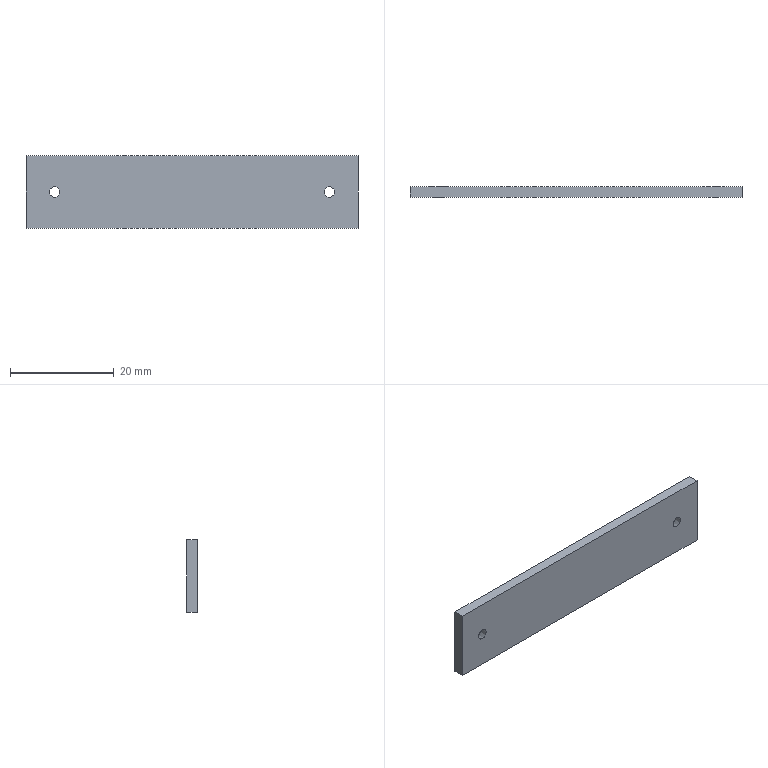Part | SolidWorks | features BaseBody 1 | 1 solid | 10 faces | box 64 x 2 x 14 mm | volume 1762 mm3 | plane 6 | cone 4
STEP:
#1=CARTESIAN_POINT('',(26.5,-1.,1.025));
#2=VERTEX_POINT('',#1);
#3=CARTESIAN_POINT('',(26.5,-1.,-1.025));
#4=VERTEX_POINT('',#3);
#5=CARTESIAN_POINT('',(26.5,-1.,0.));
#6=DIRECTION('',(0.,-1.,0.));
#7=DIRECTION('',(0.,0.,1.));
#8=AXIS2_PLACEMENT_3D('',#5,#6,#7);
#9=CIRCLE('',#8,1.025);
#10=EDGE_CURVE('',#2,#4,#9,.T.);
#11=ORIENTED_EDGE('',*,*,#10,.T.);
#12=CARTESIAN_POINT('',(26.5,1.,-2.));
#13=VERTEX_POINT('',#12);
#14=CARTESIAN_POINT('',(26.5,1.,-2.));
#15=DIRECTION('',(0.,0.8988,-0.4384));
#16=VECTOR('',#15,1000.);
#17=LINE('',#14,#16);
#18=EDGE_CURVE('',#4,#13,#17,.T.);
#19=ORIENTED_EDGE('',*,*,#18,.T.);
#20=CARTESIAN_POINT('',(26.5,1.,2.));
#21=VERTEX_POINT('',#20);
#22=CARTESIAN_POINT('',(26.5,1.,0.));
#23=DIRECTION('',(0.,-1.,0.));
#24=DIRECTION('',(0.,0.,1.));
#25=AXIS2_PLACEMENT_3D('',#22,#23,#24);
#26=CIRCLE('',#25,2.);
#27=EDGE_CURVE('',#21,#13,#26,.T.);
#28=ORIENTED_EDGE('',*,*,#27,.F.);
#29=CARTESIAN_POINT('',(26.5,1.,2.));
#30=DIRECTION('',(0.,0.8988,0.4384));
#31=VECTOR('',#30,1000.);
#32=LINE('',#29,#31);
#33=EDGE_CURVE('',#2,#21,#32,.T.);
#34=ORIENTED_EDGE('',*,*,#33,.F.);
#35=EDGE_LOOP('',(#11,#19,#28,#34));
#36=FACE_OUTER_BOUND('',#35,.T.);
#37=CARTESIAN_POINT('',(26.5,1.,0.));
#38=DIRECTION('',(0.,1.,0.));
#39=DIRECTION('',(0.,0.,1.));
#40=AXIS2_PLACEMENT_3D('',#37,#38,#39);
#41=CONICAL_SURFACE('',#40,2.,0.4538);
#42=ADVANCED_FACE('',(#36),#41,.F.);
#43=CARTESIAN_POINT('',(-26.5,-1.,1.025));
#44=VERTEX_POINT('',#43);
#45=CARTESIAN_POINT('',(-26.5,-1.,-1.025));
#46=VERTEX_POINT('',#45);
#47=CARTESIAN_POINT('',(-26.5,-1.,0.));
#48=DIRECTION('',(0.,-1.,0.));
#49=DIRECTION('',(0.,0.,1.));
#50=AXIS2_PLACEMENT_3D('',#47,#48,#49);
#51=CIRCLE('',#50,1.025);
#52=EDGE_CURVE('',#44,#46,#51,.T.);
#53=ORIENTED_EDGE('',*,*,#52,.T.);
#54=CARTESIAN_POINT('',(-26.5,1.,-2.));
#55=VERTEX_POINT('',#54);
#56=CARTESIAN_POINT('',(-26.5,1.,-2.));
#57=DIRECTION('',(0.,0.8988,-0.4384));
#58=VECTOR('',#57,1000.);
#59=LINE('',#56,#58);
#60=EDGE_CURVE('',#46,#55,#59,.T.);
#61=ORIENTED_EDGE('',*,*,#60,.T.);
#62=CARTESIAN_POINT('',(-26.5,1.,2.));
#63=VERTEX_POINT('',#62);
#64=CARTESIAN_POINT('',(-26.5,1.,0.));
#65=DIRECTION('',(0.,-1.,0.));
#66=DIRECTION('',(0.,0.,1.));
#67=AXIS2_PLACEMENT_3D('',#64,#65,#66);
#68=CIRCLE('',#67,2.);
#69=EDGE_CURVE('',#63,#55,#68,.T.);
#70=ORIENTED_EDGE('',*,*,#69,.F.);
#71=CARTESIAN_POINT('',(-26.5,1.,2.));
#72=DIRECTION('',(0.,0.8988,0.4384));
#73=VECTOR('',#72,1000.);
#74=LINE('',#71,#73);
#75=EDGE_CURVE('',#44,#63,#74,.T.);
#76=ORIENTED_EDGE('',*,*,#75,.F.);
#77=EDGE_LOOP('',(#53,#61,#70,#76));
#78=FACE_OUTER_BOUND('',#77,.T.);
#79=CARTESIAN_POINT('',(-26.5,1.,0.));
#80=DIRECTION('',(0.,1.,0.));
#81=DIRECTION('',(0.,0.,1.));
#82=AXIS2_PLACEMENT_3D('',#79,#80,#81);
#83=CONICAL_SURFACE('',#82,2.,0.4538);
#84=ADVANCED_FACE('',(#78),#83,.F.);
#85=CARTESIAN_POINT('',(32.,-1.,-7.));
#86=VERTEX_POINT('',#85);
#87=CARTESIAN_POINT('',(-32.,-1.,-7.));
#88=VERTEX_POINT('',#87);
#89=CARTESIAN_POINT('',(0.,-1.,-7.));
#90=DIRECTION('',(-1.,0.,0.));
#91=VECTOR('',#90,1000.);
#92=LINE('',#89,#91);
#93=EDGE_CURVE('',#86,#88,#92,.T.);
#94=ORIENTED_EDGE('',*,*,#93,.F.);
#95=CARTESIAN_POINT('',(32.,-1.,7.));
#96=VERTEX_POINT('',#95);
#97=CARTESIAN_POINT('',(32.,-1.,0.));
#98=DIRECTION('',(0.,0.,-1.));
#99=VECTOR('',#98,1000.);
#100=LINE('',#97,#99);
#101=EDGE_CURVE('',#96,#86,#100,.T.);
#102=ORIENTED_EDGE('',*,*,#101,.F.);
#103=CARTESIAN_POINT('',(-32.,-1.,7.));
#104=VERTEX_POINT('',#103);
#105=CARTESIAN_POINT('',(0.,-1.,7.));
#106=DIRECTION('',(1.,0.,0.));
#107=VECTOR('',#106,1000.);
#108=LINE('',#105,#107);
#109=EDGE_CURVE('',#104,#96,#108,.T.);
#110=ORIENTED_EDGE('',*,*,#109,.F.);
#111=CARTESIAN_POINT('',(-32.,-1.,0.));
#112=DIRECTION('',(0.,0.,1.));
#113=VECTOR('',#112,1000.);
#114=LINE('',#111,#113);
#115=EDGE_CURVE('',#88,#104,#114,.T.);
#116=ORIENTED_EDGE('',*,*,#115,.F.);
#117=EDGE_LOOP('',(#94,#102,#110,#116));
#118=FACE_OUTER_BOUND('',#117,.T.);
#119=ORIENTED_EDGE('',*,*,#10,.F.);
#120=CARTESIAN_POINT('',(26.5,-1.,0.));
#121=DIRECTION('',(0.,-1.,0.));
#122=DIRECTION('',(0.,0.,1.));
#123=AXIS2_PLACEMENT_3D('',#120,#121,#122);
#124=CIRCLE('',#123,1.025);
#125=EDGE_CURVE('',#4,#2,#124,.T.);
#126=ORIENTED_EDGE('',*,*,#125,.F.);
#127=EDGE_LOOP('',(#119,#126));
#128=FACE_BOUND('',#127,.T.);
#129=ORIENTED_EDGE('',*,*,#52,.F.);
#130=CARTESIAN_POINT('',(-26.5,-1.,0.));
#131=DIRECTION('',(0.,-1.,0.));
#132=DIRECTION('',(0.,0.,1.));
#133=AXIS2_PLACEMENT_3D('',#130,#131,#132);
#134=CIRCLE('',#133,1.025);
#135=EDGE_CURVE('',#46,#44,#134,.T.);
#136=ORIENTED_EDGE('',*,*,#135,.F.);
#137=EDGE_LOOP('',(#129,#136));
#138=FACE_BOUND('',#137,.T.);
#139=CARTESIAN_POINT('',(0.,-1.,0.));
#140=DIRECTION('',(0.,1.,0.));
#141=DIRECTION('',(0.,0.,1.));
#142=AXIS2_PLACEMENT_3D('',#139,#140,#141);
#143=PLANE('',#142);
#144=ADVANCED_FACE('',(#118,#128,#138),#143,.F.);
#145=CARTESIAN_POINT('',(-32.,1.,7.));
#146=VERTEX_POINT('',#145);
#147=CARTESIAN_POINT('',(-32.,1.,7.));
#148=DIRECTION('',(0.,-1.,0.));
#149=VECTOR('',#148,1000.);
#150=LINE('',#147,#149);
#151=EDGE_CURVE('',#146,#104,#150,.T.);
#152=ORIENTED_EDGE('',*,*,#151,.F.);
#153=CARTESIAN_POINT('',(-32.,1.,-7.));
#154=VERTEX_POINT('',#153);
#155=CARTESIAN_POINT('',(-32.,1.,7.));
#156=DIRECTION('',(0.,0.,1.));
#157=VECTOR('',#156,1000.);
#158=LINE('',#155,#157);
#159=EDGE_CURVE('',#154,#146,#158,.T.);
#160=ORIENTED_EDGE('',*,*,#159,.F.);
#161=CARTESIAN_POINT('',(-32.,1.,-7.));
#162=DIRECTION('',(0.,1.,0.));
#163=VECTOR('',#162,1000.);
#164=LINE('',#161,#163);
#165=EDGE_CURVE('',#88,#154,#164,.T.);
#166=ORIENTED_EDGE('',*,*,#165,.F.);
#167=ORIENTED_EDGE('',*,*,#115,.T.);
#168=EDGE_LOOP('',(#152,#160,#166,#167));
#169=FACE_OUTER_BOUND('',#168,.T.);
#170=CARTESIAN_POINT('',(-32.,1.,7.));
#171=DIRECTION('',(1.,0.,0.));
#172=DIRECTION('',(0.,0.,-1.));
#173=AXIS2_PLACEMENT_3D('',#170,#171,#172);
#174=PLANE('',#173);
#175=ADVANCED_FACE('',(#169),#174,.F.);
#176=ORIENTED_EDGE('',*,*,#165,.T.);
#177=CARTESIAN_POINT('',(32.,1.,-7.));
#178=VERTEX_POINT('',#177);
#179=CARTESIAN_POINT('',(32.,1.,-7.));
#180=DIRECTION('',(-1.,0.,0.));
#181=VECTOR('',#180,1000.);
#182=LINE('',#179,#181);
#183=EDGE_CURVE('',#178,#154,#182,.T.);
#184=ORIENTED_EDGE('',*,*,#183,.F.);
#185=CARTESIAN_POINT('',(32.,1.,-7.));
#186=DIRECTION('',(0.,1.,0.));
#187=VECTOR('',#186,1000.);
#188=LINE('',#185,#187);
#189=EDGE_CURVE('',#86,#178,#188,.T.);
#190=ORIENTED_EDGE('',*,*,#189,.F.);
#191=ORIENTED_EDGE('',*,*,#93,.T.);
#192=EDGE_LOOP('',(#176,#184,#190,#191));
#193=FACE_OUTER_BOUND('',#192,.T.);
#194=CARTESIAN_POINT('',(32.,1.,-7.));
#195=DIRECTION('',(0.,0.,1.));
#196=DIRECTION('',(1.,0.,0.));
#197=AXIS2_PLACEMENT_3D('',#194,#195,#196);
#198=PLANE('',#197);
#199=ADVANCED_FACE('',(#193),#198,.F.);
#200=ORIENTED_EDGE('',*,*,#189,.T.);
#201=CARTESIAN_POINT('',(32.,1.,7.));
#202=VERTEX_POINT('',#201);
#203=CARTESIAN_POINT('',(32.,1.,7.));
#204=DIRECTION('',(0.,0.,-1.));
#205=VECTOR('',#204,1000.);
#206=LINE('',#203,#205);
#207=EDGE_CURVE('',#202,#178,#206,.T.);
#208=ORIENTED_EDGE('',*,*,#207,.F.);
#209=CARTESIAN_POINT('',(32.,1.,7.));
#210=DIRECTION('',(0.,1.,0.));
#211=VECTOR('',#210,1000.);
#212=LINE('',#209,#211);
#213=EDGE_CURVE('',#96,#202,#212,.T.);
#214=ORIENTED_EDGE('',*,*,#213,.F.);
#215=ORIENTED_EDGE('',*,*,#101,.T.);
#216=EDGE_LOOP('',(#200,#208,#214,#215));
#217=FACE_OUTER_BOUND('',#216,.T.);
#218=CARTESIAN_POINT('',(32.,1.,7.));
#219=DIRECTION('',(-1.,0.,0.));
#220=DIRECTION('',(0.,0.,1.));
#221=AXIS2_PLACEMENT_3D('',#218,#219,#220);
#222=PLANE('',#221);
#223=ADVANCED_FACE('',(#217),#222,.F.);
#224=ORIENTED_EDGE('',*,*,#213,.T.);
#225=CARTESIAN_POINT('',(32.,1.,7.));
#226=DIRECTION('',(1.,0.,0.));
#227=VECTOR('',#226,1000.);
#228=LINE('',#225,#227);
#229=EDGE_CURVE('',#146,#202,#228,.T.);
#230=ORIENTED_EDGE('',*,*,#229,.F.);
#231=ORIENTED_EDGE('',*,*,#151,.T.);
#232=ORIENTED_EDGE('',*,*,#109,.T.);
#233=EDGE_LOOP('',(#224,#230,#231,#232));
#234=FACE_OUTER_BOUND('',#233,.T.);
#235=CARTESIAN_POINT('',(32.,1.,7.));
#236=DIRECTION('',(0.,0.,-1.));
#237=DIRECTION('',(-1.,0.,0.));
#238=AXIS2_PLACEMENT_3D('',#235,#236,#237);
#239=PLANE('',#238);
#240=ADVANCED_FACE('',(#234),#239,.F.);
#241=ORIENTED_EDGE('',*,*,#18,.F.);
#242=ORIENTED_EDGE('',*,*,#125,.T.);
#243=ORIENTED_EDGE('',*,*,#33,.T.);
#244=CARTESIAN_POINT('',(26.5,1.,0.));
#245=DIRECTION('',(0.,-1.,0.));
#246=DIRECTION('',(0.,0.,1.));
#247=AXIS2_PLACEMENT_3D('',#244,#245,#246);
#248=CIRCLE('',#247,2.);
#249=EDGE_CURVE('',#13,#21,#248,.T.);
#250=ORIENTED_EDGE('',*,*,#249,.F.);
#251=EDGE_LOOP('',(#241,#242,#243,#250));
#252=FACE_OUTER_BOUND('',#251,.T.);
#253=CARTESIAN_POINT('',(26.5,1.,0.));
#254=DIRECTION('',(0.,1.,0.));
#255=DIRECTION('',(0.,0.,1.));
#256=AXIS2_PLACEMENT_3D('',#253,#254,#255);
#257=CONICAL_SURFACE('',#256,2.,0.4538);
#258=ADVANCED_FACE('',(#252),#257,.F.);
#259=ORIENTED_EDGE('',*,*,#60,.F.);
#260=ORIENTED_EDGE('',*,*,#135,.T.);
#261=ORIENTED_EDGE('',*,*,#75,.T.);
#262=CARTESIAN_POINT('',(-26.5,1.,0.));
#263=DIRECTION('',(0.,-1.,0.));
#264=DIRECTION('',(0.,0.,1.));
#265=AXIS2_PLACEMENT_3D('',#262,#263,#264);
#266=CIRCLE('',#265,2.);
#267=EDGE_CURVE('',#55,#63,#266,.T.);
#268=ORIENTED_EDGE('',*,*,#267,.F.);
#269=EDGE_LOOP('',(#259,#260,#261,#268));
#270=FACE_OUTER_BOUND('',#269,.T.);
#271=CARTESIAN_POINT('',(-26.5,1.,0.));
#272=DIRECTION('',(0.,1.,0.));
#273=DIRECTION('',(0.,0.,1.));
#274=AXIS2_PLACEMENT_3D('',#271,#272,#273);
#275=CONICAL_SURFACE('',#274,2.,0.4538);
#276=ADVANCED_FACE('',(#270),#275,.F.);
#277=ORIENTED_EDGE('',*,*,#207,.T.);
#278=ORIENTED_EDGE('',*,*,#183,.T.);
#279=ORIENTED_EDGE('',*,*,#159,.T.);
#280=ORIENTED_EDGE('',*,*,#229,.T.);
#281=EDGE_LOOP('',(#277,#278,#279,#280));
#282=FACE_OUTER_BOUND('',#281,.T.);
#283=ORIENTED_EDGE('',*,*,#27,.T.);
#284=ORIENTED_EDGE('',*,*,#249,.T.);
#285=EDGE_LOOP('',(#283,#284));
#286=FACE_BOUND('',#285,.T.);
#287=ORIENTED_EDGE('',*,*,#69,.T.);
#288=ORIENTED_EDGE('',*,*,#267,.T.);
#289=EDGE_LOOP('',(#287,#288));
#290=FACE_BOUND('',#289,.T.);
#291=CARTESIAN_POINT('',(0.,1.,0.));
#292=DIRECTION('',(0.,1.,0.));
#293=DIRECTION('',(0.,0.,1.));
#294=AXIS2_PLACEMENT_3D('',#291,#292,#293);
#295=PLANE('',#294);
#296=ADVANCED_FACE('',(#282,#286,#290),#295,.T.);
#297=CLOSED_SHELL('',(#42,#84,#144,#175,#199,#223,#240,#258,#276,#296));
#298=MANIFOLD_SOLID_BREP('',#297);
#299=CARTESIAN_POINT('',(0.,0.,0.));
#300=DIRECTION('',(0.,0.,1.));
#301=DIRECTION('',(1.,0.,0.));
#302=AXIS2_PLACEMENT_3D('',#299,#300,#301);
#303=(LENGTH_UNIT()NAMED_UNIT(*)SI_UNIT(.MILLI.,.METRE.));
#304=UNCERTAINTY_MEASURE_WITH_UNIT(LENGTH_MEASURE(0.00001),#303,'','');
#305=(NAMED_UNIT(*)PLANE_ANGLE_UNIT()SI_UNIT($,.RADIAN.));
#306=(NAMED_UNIT(*)SI_UNIT($,.STERADIAN.)SOLID_ANGLE_UNIT());
#307=(GEOMETRIC_REPRESENTATION_CONTEXT(3)GLOBAL_UNCERTAINTY_ASSIGNED_CONTEXT((#304))GLOBAL_UNIT_ASSIGNED_CONTEXT((#303,#305,#306))REPRESENTATION_CONTEXT('',''));
#308=ADVANCED_BREP_SHAPE_REPRESENTATION('',(#298,#302),#307);